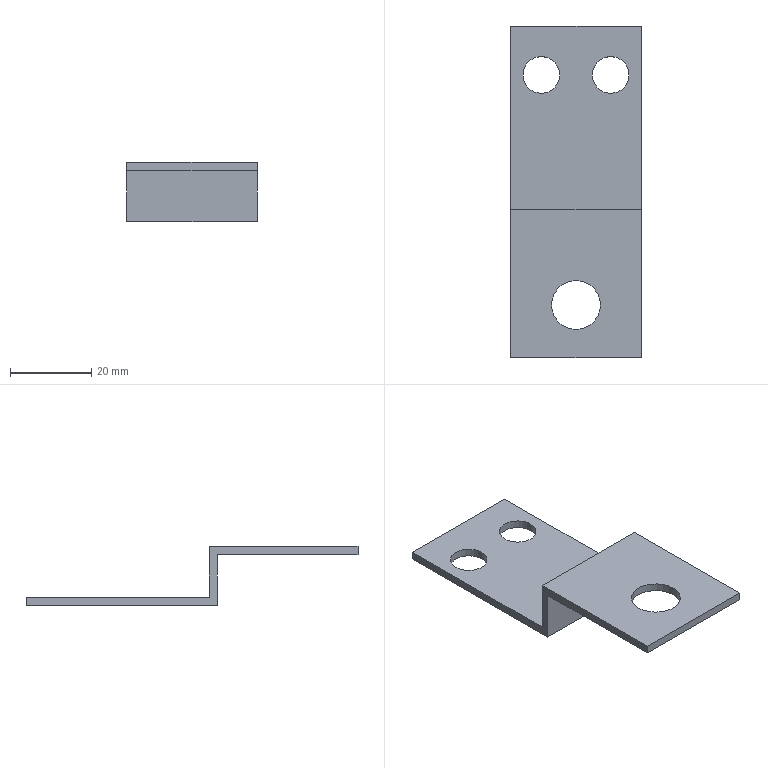Part | NX | features 20 2 | 1 solid | 13 faces | box 32 x 81.5 x 14.5 mm | volume 5535 mm3 | plane 10 | cylinder 3 | commonest cylinder face diameters 9 x2 12 x1
STEP:
#1=CARTESIAN_POINT('',(309.949,-513.5,-28.));
#2=VERTEX_POINT('',#1);
#3=CARTESIAN_POINT('',(309.949,-513.5,-40.5));
#4=VERTEX_POINT('',#3);
#5=CARTESIAN_POINT('',(309.949,-513.5,18.25));
#6=DIRECTION('',(0.,0.,-1.));
#7=VECTOR('',#6,1000.);
#8=LINE('',#5,#7);
#9=EDGE_CURVE('',#2,#4,#8,.T.);
#10=ORIENTED_EDGE('',*,*,#9,.F.);
#11=CARTESIAN_POINT('',(309.949,-548.,-28.));
#12=VERTEX_POINT('',#11);
#13=CARTESIAN_POINT('',(309.949,-534.75,-28.));
#14=DIRECTION('',(0.,1.,0.));
#15=VECTOR('',#14,1000.);
#16=LINE('',#13,#15);
#17=EDGE_CURVE('',#12,#2,#16,.T.);
#18=ORIENTED_EDGE('',*,*,#17,.F.);
#19=CARTESIAN_POINT('',(309.949,-548.,-26.));
#20=VERTEX_POINT('',#19);
#21=CARTESIAN_POINT('',(309.949,-548.,-12.5));
#22=DIRECTION('',(0.,0.,-1.));
#23=VECTOR('',#22,1000.);
#24=LINE('',#21,#23);
#25=EDGE_CURVE('',#20,#12,#24,.T.);
#26=ORIENTED_EDGE('',*,*,#25,.F.);
#27=CARTESIAN_POINT('',(309.949,-511.5,-26.));
#28=VERTEX_POINT('',#27);
#29=CARTESIAN_POINT('',(309.949,-530.,-26.));
#30=DIRECTION('',(0.,1.,0.));
#31=VECTOR('',#30,1000.);
#32=LINE('',#29,#31);
#33=EDGE_CURVE('',#20,#28,#32,.T.);
#34=ORIENTED_EDGE('',*,*,#33,.T.);
#35=CARTESIAN_POINT('',(309.949,-511.5,-38.5));
#36=VERTEX_POINT('',#35);
#37=CARTESIAN_POINT('',(309.949,-511.5,-105.5));
#38=DIRECTION('',(0.,0.,1.));
#39=VECTOR('',#38,1000.);
#40=LINE('',#37,#39);
#41=EDGE_CURVE('',#36,#28,#40,.T.);
#42=ORIENTED_EDGE('',*,*,#41,.F.);
#43=CARTESIAN_POINT('',(309.949,-466.5,-38.5));
#44=VERTEX_POINT('',#43);
#45=CARTESIAN_POINT('',(309.949,-300.5,-38.5));
#46=DIRECTION('',(0.,-1.,0.));
#47=VECTOR('',#46,1000.);
#48=LINE('',#45,#47);
#49=EDGE_CURVE('',#44,#36,#48,.T.);
#50=ORIENTED_EDGE('',*,*,#49,.F.);
#51=CARTESIAN_POINT('',(309.949,-466.5,-40.5));
#52=VERTEX_POINT('',#51);
#53=CARTESIAN_POINT('',(309.949,-466.5,-70.));
#54=DIRECTION('',(0.,0.,1.));
#55=VECTOR('',#54,1000.);
#56=LINE('',#53,#55);
#57=EDGE_CURVE('',#52,#44,#56,.T.);
#58=ORIENTED_EDGE('',*,*,#57,.F.);
#59=CARTESIAN_POINT('',(309.949,-300.5,-40.5));
#60=DIRECTION('',(0.,1.,0.));
#61=VECTOR('',#60,1000.);
#62=LINE('',#59,#61);
#63=EDGE_CURVE('',#4,#52,#62,.T.);
#64=ORIENTED_EDGE('',*,*,#63,.F.);
#65=EDGE_LOOP('',(#10,#18,#26,#34,#42,#50,#58,#64));
#66=FACE_BOUND('',#65,.T.);
#67=CARTESIAN_POINT('',(309.949,-530.,99.5));
#68=DIRECTION('',(-1.,0.,0.));
#69=DIRECTION('',(0.,-1.,0.));
#70=AXIS2_PLACEMENT_3D('',#67,#68,#69);
#71=PLANE('',#70);
#72=ADVANCED_FACE('',(#66),#71,.T.);
#73=CARTESIAN_POINT('',(341.949,-548.,-26.));
#74=VERTEX_POINT('',#73);
#75=CARTESIAN_POINT('',(341.949,-511.5,-26.));
#76=VERTEX_POINT('',#75);
#77=CARTESIAN_POINT('',(341.949,-530.,-26.));
#78=DIRECTION('',(0.,1.,0.));
#79=VECTOR('',#78,1000.);
#80=LINE('',#77,#79);
#81=EDGE_CURVE('',#74,#76,#80,.T.);
#82=ORIENTED_EDGE('',*,*,#81,.F.);
#83=CARTESIAN_POINT('',(341.949,-548.,-28.));
#84=VERTEX_POINT('',#83);
#85=CARTESIAN_POINT('',(341.949,-548.,-12.5));
#86=DIRECTION('',(0.,0.,1.));
#87=VECTOR('',#86,1000.);
#88=LINE('',#85,#87);
#89=EDGE_CURVE('',#84,#74,#88,.T.);
#90=ORIENTED_EDGE('',*,*,#89,.F.);
#91=CARTESIAN_POINT('',(341.949,-513.5,-28.));
#92=VERTEX_POINT('',#91);
#93=CARTESIAN_POINT('',(341.949,-530.,-28.));
#94=DIRECTION('',(0.,-1.,0.));
#95=VECTOR('',#94,1000.);
#96=LINE('',#93,#95);
#97=EDGE_CURVE('',#92,#84,#96,.T.);
#98=ORIENTED_EDGE('',*,*,#97,.F.);
#99=CARTESIAN_POINT('',(341.949,-513.5,-40.5));
#100=VERTEX_POINT('',#99);
#101=CARTESIAN_POINT('',(341.949,-513.5,99.5));
#102=DIRECTION('',(0.,0.,1.));
#103=VECTOR('',#102,1000.);
#104=LINE('',#101,#103);
#105=EDGE_CURVE('',#100,#92,#104,.T.);
#106=ORIENTED_EDGE('',*,*,#105,.F.);
#107=CARTESIAN_POINT('',(341.949,-466.5,-40.5));
#108=VERTEX_POINT('',#107);
#109=CARTESIAN_POINT('',(341.949,-530.,-40.5));
#110=DIRECTION('',(0.,-1.,0.));
#111=VECTOR('',#110,1000.);
#112=LINE('',#109,#111);
#113=EDGE_CURVE('',#108,#100,#112,.T.);
#114=ORIENTED_EDGE('',*,*,#113,.F.);
#115=CARTESIAN_POINT('',(341.949,-466.5,-38.5));
#116=VERTEX_POINT('',#115);
#117=CARTESIAN_POINT('',(341.949,-466.5,-70.));
#118=DIRECTION('',(0.,0.,-1.));
#119=VECTOR('',#118,1000.);
#120=LINE('',#117,#119);
#121=EDGE_CURVE('',#116,#108,#120,.T.);
#122=ORIENTED_EDGE('',*,*,#121,.F.);
#123=CARTESIAN_POINT('',(341.949,-511.5,-38.5));
#124=VERTEX_POINT('',#123);
#125=CARTESIAN_POINT('',(341.949,-530.,-38.5));
#126=DIRECTION('',(0.,1.,0.));
#127=VECTOR('',#126,1000.);
#128=LINE('',#125,#127);
#129=EDGE_CURVE('',#124,#116,#128,.T.);
#130=ORIENTED_EDGE('',*,*,#129,.F.);
#131=CARTESIAN_POINT('',(341.949,-511.5,99.5));
#132=DIRECTION('',(0.,0.,1.));
#133=VECTOR('',#132,1000.);
#134=LINE('',#131,#133);
#135=EDGE_CURVE('',#124,#76,#134,.T.);
#136=ORIENTED_EDGE('',*,*,#135,.T.);
#137=EDGE_LOOP('',(#82,#90,#98,#106,#114,#122,#130,#136));
#138=FACE_BOUND('',#137,.T.);
#139=CARTESIAN_POINT('',(341.949,-530.,99.5));
#140=DIRECTION('',(-1.,0.,0.));
#141=DIRECTION('',(0.,-1.,0.));
#142=AXIS2_PLACEMENT_3D('',#139,#140,#141);
#143=PLANE('',#142);
#144=ADVANCED_FACE('',(#138),#143,.F.);
#145=CARTESIAN_POINT('',(324.949,-513.5,-28.));
#146=DIRECTION('',(1.,0.,0.));
#147=VECTOR('',#146,1000.);
#148=LINE('',#145,#147);
#149=EDGE_CURVE('',#2,#92,#148,.T.);
#150=ORIENTED_EDGE('',*,*,#149,.F.);
#151=ORIENTED_EDGE('',*,*,#9,.T.);
#152=CARTESIAN_POINT('',(424.5,-513.5,-40.5));
#153=DIRECTION('',(-1.,0.,0.));
#154=VECTOR('',#153,1000.);
#155=LINE('',#152,#154);
#156=EDGE_CURVE('',#100,#4,#155,.T.);
#157=ORIENTED_EDGE('',*,*,#156,.F.);
#158=ORIENTED_EDGE('',*,*,#105,.T.);
#159=EDGE_LOOP('',(#150,#151,#157,#158));
#160=FACE_BOUND('',#159,.T.);
#161=CARTESIAN_POINT('',(324.949,-513.5,18.25));
#162=DIRECTION('',(0.,-1.,0.));
#163=DIRECTION('',(0.,0.,1.));
#164=AXIS2_PLACEMENT_3D('',#161,#162,#163);
#165=PLANE('',#164);
#166=ADVANCED_FACE('',(#160),#165,.T.);
#167=ORIENTED_EDGE('',*,*,#41,.T.);
#168=CARTESIAN_POINT('',(406.448,-511.5,-26.));
#169=DIRECTION('',(-1.,0.,0.));
#170=VECTOR('',#169,1000.);
#171=LINE('',#168,#170);
#172=EDGE_CURVE('',#76,#28,#171,.T.);
#173=ORIENTED_EDGE('',*,*,#172,.F.);
#174=ORIENTED_EDGE('',*,*,#135,.F.);
#175=CARTESIAN_POINT('',(424.5,-511.5,-38.5));
#176=DIRECTION('',(-1.,0.,0.));
#177=VECTOR('',#176,1000.);
#178=LINE('',#175,#177);
#179=EDGE_CURVE('',#124,#36,#178,.T.);
#180=ORIENTED_EDGE('',*,*,#179,.T.);
#181=EDGE_LOOP('',(#167,#173,#174,#180));
#182=FACE_BOUND('',#181,.T.);
#183=CARTESIAN_POINT('',(406.448,-511.5,-105.5));
#184=DIRECTION('',(0.,1.,0.));
#185=DIRECTION('',(0.,0.,-1.));
#186=AXIS2_PLACEMENT_3D('',#183,#184,#185);
#187=PLANE('',#186);
#188=ADVANCED_FACE('',(#182),#187,.T.);
#189=CARTESIAN_POINT('',(325.949,-466.5,-40.5));
#190=DIRECTION('',(1.,0.,0.));
#191=VECTOR('',#190,1000.);
#192=LINE('',#189,#191);
#193=EDGE_CURVE('',#52,#108,#192,.T.);
#194=ORIENTED_EDGE('',*,*,#193,.T.);
#195=ORIENTED_EDGE('',*,*,#113,.T.);
#196=ORIENTED_EDGE('',*,*,#156,.T.);
#197=ORIENTED_EDGE('',*,*,#63,.T.);
#198=EDGE_LOOP('',(#194,#195,#196,#197));
#199=FACE_BOUND('',#198,.T.);
#200=CARTESIAN_POINT('',(312.949,-478.5,-40.5));
#201=VERTEX_POINT('',#200);
#202=CARTESIAN_POINT('',(317.449,-478.5,-40.5));
#203=DIRECTION('',(0.,0.,1.));
#204=DIRECTION('',(-1.,0.,0.));
#205=AXIS2_PLACEMENT_3D('',#202,#203,#204);
#206=CIRCLE('',#205,4.5);
#207=EDGE_CURVE('',#201,#201,#206,.T.);
#208=ORIENTED_EDGE('',*,*,#207,.T.);
#209=EDGE_LOOP('',(#208));
#210=FACE_BOUND('',#209,.T.);
#211=CARTESIAN_POINT('',(329.949,-478.5,-40.5));
#212=VERTEX_POINT('',#211);
#213=CARTESIAN_POINT('',(334.449,-478.5,-40.5));
#214=DIRECTION('',(0.,0.,-1.));
#215=DIRECTION('',(-1.,0.,0.));
#216=AXIS2_PLACEMENT_3D('',#213,#214,#215);
#217=CIRCLE('',#216,4.5);
#218=EDGE_CURVE('',#212,#212,#217,.T.);
#219=ORIENTED_EDGE('',*,*,#218,.F.);
#220=EDGE_LOOP('',(#219));
#221=FACE_BOUND('',#220,.T.);
#222=CARTESIAN_POINT('',(424.5,-300.5,-40.5));
#223=DIRECTION('',(0.,0.,-1.));
#224=DIRECTION('',(-1.,0.,0.));
#225=AXIS2_PLACEMENT_3D('',#222,#223,#224);
#226=PLANE('',#225);
#227=ADVANCED_FACE('',(#199,#210,#221),#226,.T.);
#228=ORIENTED_EDGE('',*,*,#179,.F.);
#229=ORIENTED_EDGE('',*,*,#129,.T.);
#230=CARTESIAN_POINT('',(325.949,-466.5,-38.5));
#231=DIRECTION('',(-1.,0.,0.));
#232=VECTOR('',#231,1000.);
#233=LINE('',#230,#232);
#234=EDGE_CURVE('',#116,#44,#233,.T.);
#235=ORIENTED_EDGE('',*,*,#234,.T.);
#236=ORIENTED_EDGE('',*,*,#49,.T.);
#237=EDGE_LOOP('',(#228,#229,#235,#236));
#238=FACE_BOUND('',#237,.T.);
#239=CARTESIAN_POINT('',(329.949,-478.5,-38.5));
#240=VERTEX_POINT('',#239);
#241=CARTESIAN_POINT('',(334.449,-478.5,-38.5));
#242=DIRECTION('',(0.,0.,1.));
#243=DIRECTION('',(-1.,0.,0.));
#244=AXIS2_PLACEMENT_3D('',#241,#242,#243);
#245=CIRCLE('',#244,4.5);
#246=EDGE_CURVE('',#240,#240,#245,.T.);
#247=ORIENTED_EDGE('',*,*,#246,.F.);
#248=EDGE_LOOP('',(#247));
#249=FACE_BOUND('',#248,.T.);
#250=CARTESIAN_POINT('',(312.949,-478.5,-38.5));
#251=VERTEX_POINT('',#250);
#252=CARTESIAN_POINT('',(317.449,-478.5,-38.5));
#253=DIRECTION('',(0.,0.,1.));
#254=DIRECTION('',(-1.,0.,0.));
#255=AXIS2_PLACEMENT_3D('',#252,#253,#254);
#256=CIRCLE('',#255,4.5);
#257=EDGE_CURVE('',#251,#251,#256,.T.);
#258=ORIENTED_EDGE('',*,*,#257,.F.);
#259=EDGE_LOOP('',(#258));
#260=FACE_BOUND('',#259,.T.);
#261=CARTESIAN_POINT('',(424.5,-300.5,-38.5));
#262=DIRECTION('',(0.,0.,-1.));
#263=DIRECTION('',(-1.,0.,0.));
#264=AXIS2_PLACEMENT_3D('',#261,#262,#263);
#265=PLANE('',#264);
#266=ADVANCED_FACE('',(#238,#249,#260),#265,.F.);
#267=ORIENTED_EDGE('',*,*,#246,.T.);
#268=EDGE_LOOP('',(#267));
#269=FACE_BOUND('',#268,.T.);
#270=ORIENTED_EDGE('',*,*,#218,.T.);
#271=EDGE_LOOP('',(#270));
#272=FACE_BOUND('',#271,.T.);
#273=CARTESIAN_POINT('',(334.449,-478.5,-35.));
#274=DIRECTION('',(0.,0.,1.));
#275=DIRECTION('',(1.,0.,0.));
#276=AXIS2_PLACEMENT_3D('',#273,#274,#275);
#277=CYLINDRICAL_SURFACE('',#276,4.5);
#278=ADVANCED_FACE('',(#269,#272),#277,.F.);
#279=ORIENTED_EDGE('',*,*,#257,.T.);
#280=EDGE_LOOP('',(#279));
#281=FACE_BOUND('',#280,.T.);
#282=ORIENTED_EDGE('',*,*,#207,.F.);
#283=EDGE_LOOP('',(#282));
#284=FACE_BOUND('',#283,.T.);
#285=CARTESIAN_POINT('',(317.449,-478.5,-35.));
#286=DIRECTION('',(0.,0.,1.));
#287=DIRECTION('',(-1.,0.,0.));
#288=AXIS2_PLACEMENT_3D('',#285,#286,#287);
#289=CYLINDRICAL_SURFACE('',#288,4.5);
#290=ADVANCED_FACE('',(#281,#284),#289,.F.);
#291=ORIENTED_EDGE('',*,*,#121,.T.);
#292=ORIENTED_EDGE('',*,*,#193,.F.);
#293=ORIENTED_EDGE('',*,*,#57,.T.);
#294=ORIENTED_EDGE('',*,*,#234,.F.);
#295=EDGE_LOOP('',(#291,#292,#293,#294));
#296=FACE_BOUND('',#295,.T.);
#297=CARTESIAN_POINT('',(325.949,-466.5,-60.75));
#298=DIRECTION('',(0.,-1.,0.));
#299=DIRECTION('',(-1.,0.,0.));
#300=AXIS2_PLACEMENT_3D('',#297,#298,#299);
#301=PLANE('',#300);
#302=ADVANCED_FACE('',(#296),#301,.F.);
#303=ORIENTED_EDGE('',*,*,#33,.F.);
#304=CARTESIAN_POINT('',(328.448,-548.,-26.));
#305=DIRECTION('',(-1.,0.,0.));
#306=VECTOR('',#305,1000.);
#307=LINE('',#304,#306);
#308=EDGE_CURVE('',#74,#20,#307,.T.);
#309=ORIENTED_EDGE('',*,*,#308,.F.);
#310=ORIENTED_EDGE('',*,*,#81,.T.);
#311=ORIENTED_EDGE('',*,*,#172,.T.);
#312=EDGE_LOOP('',(#303,#309,#310,#311));
#313=FACE_BOUND('',#312,.T.);
#314=CARTESIAN_POINT('',(331.949,-535.,-26.));
#315=VERTEX_POINT('',#314);
#316=CARTESIAN_POINT('',(325.949,-535.,-26.));
#317=DIRECTION('',(0.,0.,1.));
#318=DIRECTION('',(1.,0.,0.));
#319=AXIS2_PLACEMENT_3D('',#316,#317,#318);
#320=CIRCLE('',#319,6.);
#321=EDGE_CURVE('',#315,#315,#320,.T.);
#322=ORIENTED_EDGE('',*,*,#321,.F.);
#323=EDGE_LOOP('',(#322));
#324=FACE_BOUND('',#323,.T.);
#325=CARTESIAN_POINT('',(406.448,-411.,-26.));
#326=DIRECTION('',(0.,0.,1.));
#327=DIRECTION('',(0.,1.,0.));
#328=AXIS2_PLACEMENT_3D('',#325,#326,#327);
#329=PLANE('',#328);
#330=ADVANCED_FACE('',(#313,#324),#329,.T.);
#331=ORIENTED_EDGE('',*,*,#321,.T.);
#332=EDGE_LOOP('',(#331));
#333=FACE_BOUND('',#332,.T.);
#334=CARTESIAN_POINT('',(319.949,-535.,-28.));
#335=VERTEX_POINT('',#334);
#336=CARTESIAN_POINT('',(325.949,-535.,-28.));
#337=DIRECTION('',(0.,0.,1.));
#338=DIRECTION('',(-1.,0.,0.));
#339=AXIS2_PLACEMENT_3D('',#336,#337,#338);
#340=CIRCLE('',#339,6.);
#341=EDGE_CURVE('',#335,#335,#340,.T.);
#342=ORIENTED_EDGE('',*,*,#341,.F.);
#343=EDGE_LOOP('',(#342));
#344=FACE_BOUND('',#343,.T.);
#345=CARTESIAN_POINT('',(325.949,-535.,37.356));
#346=DIRECTION('',(0.,-0.000000114,-1.));
#347=DIRECTION('',(0.,-1.,0.000000114));
#348=AXIS2_PLACEMENT_3D('',#345,#346,#347);
#349=CYLINDRICAL_SURFACE('',#348,6.);
#350=ADVANCED_FACE('',(#333,#344),#349,.F.);
#351=CARTESIAN_POINT('',(324.949,-548.,-28.));
#352=DIRECTION('',(-1.,0.,0.));
#353=VECTOR('',#352,1000.);
#354=LINE('',#351,#353);
#355=EDGE_CURVE('',#84,#12,#354,.T.);
#356=ORIENTED_EDGE('',*,*,#355,.F.);
#357=ORIENTED_EDGE('',*,*,#89,.T.);
#358=ORIENTED_EDGE('',*,*,#308,.T.);
#359=ORIENTED_EDGE('',*,*,#25,.T.);
#360=EDGE_LOOP('',(#356,#357,#358,#359));
#361=FACE_BOUND('',#360,.T.);
#362=CARTESIAN_POINT('',(328.448,-548.,-12.5));
#363=DIRECTION('',(0.,-1.,0.));
#364=DIRECTION('',(-1.,0.,0.));
#365=AXIS2_PLACEMENT_3D('',#362,#363,#364);
#366=PLANE('',#365);
#367=ADVANCED_FACE('',(#361),#366,.T.);
#368=ORIENTED_EDGE('',*,*,#149,.T.);
#369=ORIENTED_EDGE('',*,*,#97,.T.);
#370=ORIENTED_EDGE('',*,*,#355,.T.);
#371=ORIENTED_EDGE('',*,*,#17,.T.);
#372=EDGE_LOOP('',(#368,#369,#370,#371));
#373=FACE_BOUND('',#372,.T.);
#374=ORIENTED_EDGE('',*,*,#341,.T.);
#375=EDGE_LOOP('',(#374));
#376=FACE_BOUND('',#375,.T.);
#377=CARTESIAN_POINT('',(324.949,-534.75,-28.));
#378=DIRECTION('',(0.,0.,-1.));
#379=DIRECTION('',(0.,-1.,0.));
#380=AXIS2_PLACEMENT_3D('',#377,#378,#379);
#381=PLANE('',#380);
#382=ADVANCED_FACE('',(#373,#376),#381,.T.);
#383=CLOSED_SHELL('',(#72,#144,#166,#188,#227,#266,#278,#290,#302,#330,#350,#367,#382));
#384=MANIFOLD_SOLID_BREP('',#383);
#385=(LENGTH_UNIT()NAMED_UNIT(*)SI_UNIT(.MILLI.,.METRE.));
#386=UNCERTAINTY_MEASURE_WITH_UNIT(LENGTH_MEASURE(0.00001),#385,'','');
#387=(NAMED_UNIT(*)PLANE_ANGLE_UNIT()SI_UNIT($,.RADIAN.));
#388=(NAMED_UNIT(*)SI_UNIT($,.STERADIAN.)SOLID_ANGLE_UNIT());
#389=(GEOMETRIC_REPRESENTATION_CONTEXT(3)GLOBAL_UNCERTAINTY_ASSIGNED_CONTEXT((#386))GLOBAL_UNIT_ASSIGNED_CONTEXT((#385,#387,#388))REPRESENTATION_CONTEXT('',''));
#390=ADVANCED_BREP_SHAPE_REPRESENTATION('',(#384),#389);